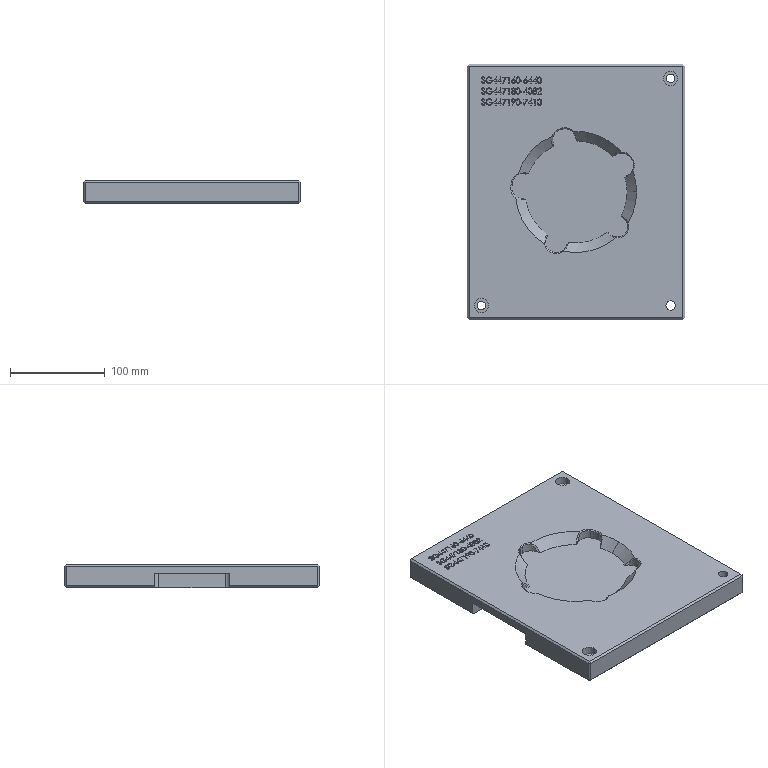Part | STEP file | 10P30 assy jig base | 1 solid | 583 faces | box 230 x 270 x 25 mm | volume 1350745 mm3 | plane 324 | spline 203 | cylinder 30 | cone 26 | commonest cylinder face diameters 22 x13 10 x6 9 x4 15 x4 136 x3